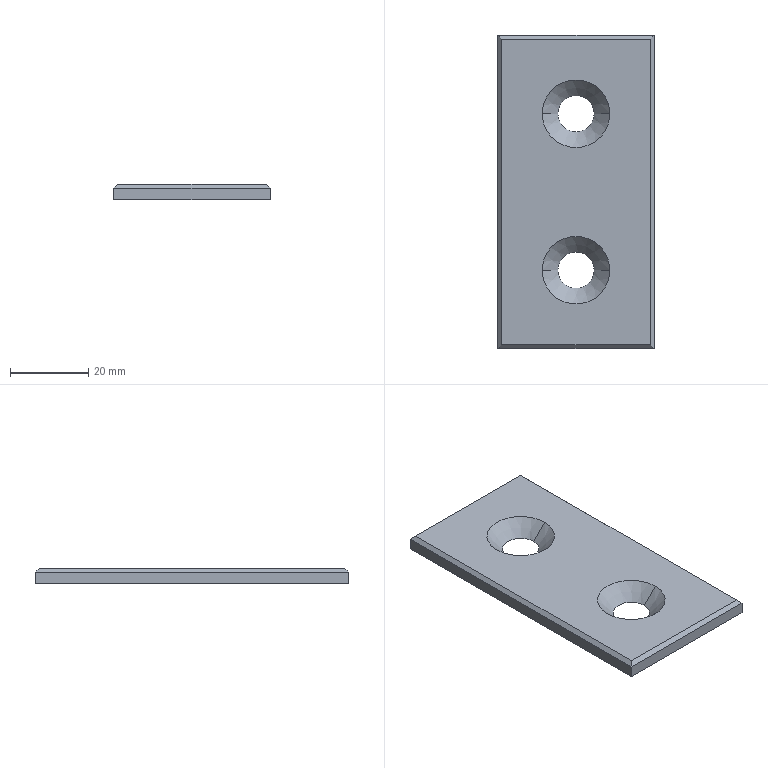Part | SolidWorks | features 3DProfileFeature 1, Chamfer 1, Extrusion 1, HoleWzd 1 | 1 solid | 14 faces | box 40 x 80 x 4 mm | volume 11536 mm3 | plane 10 | cone 4
STEP:
#1=CARTESIAN_POINT('',(-4.65,20.,-2.));
#2=VERTEX_POINT('',#1);
#3=CARTESIAN_POINT('',(4.65,20.,-2.));
#4=VERTEX_POINT('',#3);
#5=CARTESIAN_POINT('',(0.,20.,-2.));
#6=DIRECTION('',(0.,0.,1.));
#7=DIRECTION('',(1.,0.,0.));
#8=AXIS2_PLACEMENT_3D('',#5,#6,#7);
#9=CIRCLE('',#8,4.65);
#10=EDGE_CURVE('',#2,#4,#9,.T.);
#11=ORIENTED_EDGE('',*,*,#10,.F.);
#12=CARTESIAN_POINT('',(-8.65,20.,2.));
#13=VERTEX_POINT('',#12);
#14=CARTESIAN_POINT('',(-8.65,20.,2.));
#15=DIRECTION('',(-0.7071,0.,0.7071));
#16=VECTOR('',#15,1000.);
#17=LINE('',#14,#16);
#18=EDGE_CURVE('',#2,#13,#17,.T.);
#19=ORIENTED_EDGE('',*,*,#18,.T.);
#20=CARTESIAN_POINT('',(8.65,20.,2.));
#21=VERTEX_POINT('',#20);
#22=CARTESIAN_POINT('',(0.,20.,2.));
#23=DIRECTION('',(0.,0.,1.));
#24=DIRECTION('',(1.,0.,0.));
#25=AXIS2_PLACEMENT_3D('',#22,#23,#24);
#26=CIRCLE('',#25,8.65);
#27=EDGE_CURVE('',#13,#21,#26,.T.);
#28=ORIENTED_EDGE('',*,*,#27,.T.);
#29=CARTESIAN_POINT('',(8.65,20.,2.));
#30=DIRECTION('',(0.7071,0.,0.7071));
#31=VECTOR('',#30,1000.);
#32=LINE('',#29,#31);
#33=EDGE_CURVE('',#4,#21,#32,.T.);
#34=ORIENTED_EDGE('',*,*,#33,.F.);
#35=EDGE_LOOP('',(#11,#19,#28,#34));
#36=FACE_OUTER_BOUND('',#35,.T.);
#37=CARTESIAN_POINT('',(0.,20.,2.));
#38=DIRECTION('',(0.,0.,1.));
#39=DIRECTION('',(1.,0.,0.));
#40=AXIS2_PLACEMENT_3D('',#37,#38,#39);
#41=CONICAL_SURFACE('',#40,8.65,0.7854);
#42=ADVANCED_FACE('',(#36),#41,.F.);
#43=CARTESIAN_POINT('',(-4.65,-20.,-2.));
#44=VERTEX_POINT('',#43);
#45=CARTESIAN_POINT('',(4.65,-20.,-2.));
#46=VERTEX_POINT('',#45);
#47=CARTESIAN_POINT('',(0.,-20.,-2.));
#48=DIRECTION('',(0.,0.,1.));
#49=DIRECTION('',(1.,0.,0.));
#50=AXIS2_PLACEMENT_3D('',#47,#48,#49);
#51=CIRCLE('',#50,4.65);
#52=EDGE_CURVE('',#44,#46,#51,.T.);
#53=ORIENTED_EDGE('',*,*,#52,.F.);
#54=CARTESIAN_POINT('',(-8.65,-20.,2.));
#55=VERTEX_POINT('',#54);
#56=CARTESIAN_POINT('',(-8.65,-20.,2.));
#57=DIRECTION('',(-0.7071,0.,0.7071));
#58=VECTOR('',#57,1000.);
#59=LINE('',#56,#58);
#60=EDGE_CURVE('',#44,#55,#59,.T.);
#61=ORIENTED_EDGE('',*,*,#60,.T.);
#62=CARTESIAN_POINT('',(8.65,-20.,2.));
#63=VERTEX_POINT('',#62);
#64=CARTESIAN_POINT('',(0.,-20.,2.));
#65=DIRECTION('',(0.,0.,1.));
#66=DIRECTION('',(1.,0.,0.));
#67=AXIS2_PLACEMENT_3D('',#64,#65,#66);
#68=CIRCLE('',#67,8.65);
#69=EDGE_CURVE('',#55,#63,#68,.T.);
#70=ORIENTED_EDGE('',*,*,#69,.T.);
#71=CARTESIAN_POINT('',(8.65,-20.,2.));
#72=DIRECTION('',(0.7071,0.,0.7071));
#73=VECTOR('',#72,1000.);
#74=LINE('',#71,#73);
#75=EDGE_CURVE('',#46,#63,#74,.T.);
#76=ORIENTED_EDGE('',*,*,#75,.F.);
#77=EDGE_LOOP('',(#53,#61,#70,#76));
#78=FACE_OUTER_BOUND('',#77,.T.);
#79=CARTESIAN_POINT('',(0.,-20.,2.));
#80=DIRECTION('',(0.,0.,1.));
#81=DIRECTION('',(1.,0.,0.));
#82=AXIS2_PLACEMENT_3D('',#79,#80,#81);
#83=CONICAL_SURFACE('',#82,8.65,0.7854);
#84=ADVANCED_FACE('',(#78),#83,.F.);
#85=CARTESIAN_POINT('',(20.,40.,1.));
#86=VERTEX_POINT('',#85);
#87=CARTESIAN_POINT('',(20.,40.,-2.));
#88=VERTEX_POINT('',#87);
#89=CARTESIAN_POINT('',(20.,40.,2.));
#90=DIRECTION('',(0.,0.,-1.));
#91=VECTOR('',#90,1000.);
#92=LINE('',#89,#91);
#93=EDGE_CURVE('',#86,#88,#92,.T.);
#94=ORIENTED_EDGE('',*,*,#93,.F.);
#95=CARTESIAN_POINT('',(20.,-40.,1.));
#96=VERTEX_POINT('',#95);
#97=CARTESIAN_POINT('',(20.,-40.,1.));
#98=DIRECTION('',(0.,-1.,0.));
#99=VECTOR('',#98,1000.);
#100=LINE('',#97,#99);
#101=EDGE_CURVE('',#86,#96,#100,.T.);
#102=ORIENTED_EDGE('',*,*,#101,.T.);
#103=CARTESIAN_POINT('',(20.,-40.,-2.));
#104=VERTEX_POINT('',#103);
#105=CARTESIAN_POINT('',(20.,-40.,2.));
#106=DIRECTION('',(0.,0.,-1.));
#107=VECTOR('',#106,1000.);
#108=LINE('',#105,#107);
#109=EDGE_CURVE('',#96,#104,#108,.T.);
#110=ORIENTED_EDGE('',*,*,#109,.T.);
#111=CARTESIAN_POINT('',(20.,40.,-2.));
#112=DIRECTION('',(0.,1.,0.));
#113=VECTOR('',#112,1000.);
#114=LINE('',#111,#113);
#115=EDGE_CURVE('',#104,#88,#114,.T.);
#116=ORIENTED_EDGE('',*,*,#115,.T.);
#117=EDGE_LOOP('',(#94,#102,#110,#116));
#118=FACE_OUTER_BOUND('',#117,.T.);
#119=CARTESIAN_POINT('',(20.,40.,2.));
#120=DIRECTION('',(-1.,0.,0.));
#121=DIRECTION('',(0.,-1.,0.));
#122=AXIS2_PLACEMENT_3D('',#119,#120,#121);
#123=PLANE('',#122);
#124=ADVANCED_FACE('',(#118),#123,.F.);
#125=CARTESIAN_POINT('',(-20.,40.,1.));
#126=VERTEX_POINT('',#125);
#127=CARTESIAN_POINT('',(-20.,40.,-2.));
#128=VERTEX_POINT('',#127);
#129=CARTESIAN_POINT('',(-20.,40.,2.));
#130=DIRECTION('',(0.,0.,-1.));
#131=VECTOR('',#130,1000.);
#132=LINE('',#129,#131);
#133=EDGE_CURVE('',#126,#128,#132,.T.);
#134=ORIENTED_EDGE('',*,*,#133,.F.);
#135=CARTESIAN_POINT('',(20.,40.,1.));
#136=DIRECTION('',(1.,0.,0.));
#137=VECTOR('',#136,1000.);
#138=LINE('',#135,#137);
#139=EDGE_CURVE('',#126,#86,#138,.T.);
#140=ORIENTED_EDGE('',*,*,#139,.T.);
#141=ORIENTED_EDGE('',*,*,#93,.T.);
#142=CARTESIAN_POINT('',(-20.,40.,-2.));
#143=DIRECTION('',(-1.,0.,0.));
#144=VECTOR('',#143,1000.);
#145=LINE('',#142,#144);
#146=EDGE_CURVE('',#88,#128,#145,.T.);
#147=ORIENTED_EDGE('',*,*,#146,.T.);
#148=EDGE_LOOP('',(#134,#140,#141,#147));
#149=FACE_OUTER_BOUND('',#148,.T.);
#150=CARTESIAN_POINT('',(-20.,40.,2.));
#151=DIRECTION('',(0.,-1.,0.));
#152=DIRECTION('',(0.,0.,-1.));
#153=AXIS2_PLACEMENT_3D('',#150,#151,#152);
#154=PLANE('',#153);
#155=ADVANCED_FACE('',(#149),#154,.F.);
#156=CARTESIAN_POINT('',(-20.,-40.,1.));
#157=VERTEX_POINT('',#156);
#158=CARTESIAN_POINT('',(-20.,-40.,-2.));
#159=VERTEX_POINT('',#158);
#160=CARTESIAN_POINT('',(-20.,-40.,2.));
#161=DIRECTION('',(0.,0.,-1.));
#162=VECTOR('',#161,1000.);
#163=LINE('',#160,#162);
#164=EDGE_CURVE('',#157,#159,#163,.T.);
#165=ORIENTED_EDGE('',*,*,#164,.F.);
#166=CARTESIAN_POINT('',(-20.,40.,1.));
#167=DIRECTION('',(0.,1.,0.));
#168=VECTOR('',#167,1000.);
#169=LINE('',#166,#168);
#170=EDGE_CURVE('',#157,#126,#169,.T.);
#171=ORIENTED_EDGE('',*,*,#170,.T.);
#172=ORIENTED_EDGE('',*,*,#133,.T.);
#173=CARTESIAN_POINT('',(-20.,40.,-2.));
#174=DIRECTION('',(0.,-1.,0.));
#175=VECTOR('',#174,1000.);
#176=LINE('',#173,#175);
#177=EDGE_CURVE('',#128,#159,#176,.T.);
#178=ORIENTED_EDGE('',*,*,#177,.T.);
#179=EDGE_LOOP('',(#165,#171,#172,#178));
#180=FACE_OUTER_BOUND('',#179,.T.);
#181=CARTESIAN_POINT('',(-20.,40.,2.));
#182=DIRECTION('',(1.,0.,0.));
#183=DIRECTION('',(0.,1.,0.));
#184=AXIS2_PLACEMENT_3D('',#181,#182,#183);
#185=PLANE('',#184);
#186=ADVANCED_FACE('',(#180),#185,.F.);
#187=ORIENTED_EDGE('',*,*,#109,.F.);
#188=CARTESIAN_POINT('',(-20.,-40.,1.));
#189=DIRECTION('',(-1.,0.,0.));
#190=VECTOR('',#189,1000.);
#191=LINE('',#188,#190);
#192=EDGE_CURVE('',#96,#157,#191,.T.);
#193=ORIENTED_EDGE('',*,*,#192,.T.);
#194=ORIENTED_EDGE('',*,*,#164,.T.);
#195=CARTESIAN_POINT('',(-20.,-40.,-2.));
#196=DIRECTION('',(1.,0.,0.));
#197=VECTOR('',#196,1000.);
#198=LINE('',#195,#197);
#199=EDGE_CURVE('',#159,#104,#198,.T.);
#200=ORIENTED_EDGE('',*,*,#199,.T.);
#201=EDGE_LOOP('',(#187,#193,#194,#200));
#202=FACE_OUTER_BOUND('',#201,.T.);
#203=CARTESIAN_POINT('',(-20.,-40.,2.));
#204=DIRECTION('',(0.,1.,0.));
#205=DIRECTION('',(0.,0.,1.));
#206=AXIS2_PLACEMENT_3D('',#203,#204,#205);
#207=PLANE('',#206);
#208=ADVANCED_FACE('',(#202),#207,.F.);
#209=CARTESIAN_POINT('',(-19.,39.,2.));
#210=VERTEX_POINT('',#209);
#211=CARTESIAN_POINT('',(-19.,-39.,2.));
#212=VERTEX_POINT('',#211);
#213=CARTESIAN_POINT('',(-19.,-40.,2.));
#214=DIRECTION('',(0.,-1.,0.));
#215=VECTOR('',#214,1000.);
#216=LINE('',#213,#215);
#217=EDGE_CURVE('',#210,#212,#216,.T.);
#218=ORIENTED_EDGE('',*,*,#217,.T.);
#219=CARTESIAN_POINT('',(19.,-39.,2.));
#220=VERTEX_POINT('',#219);
#221=CARTESIAN_POINT('',(20.,-39.,2.));
#222=DIRECTION('',(1.,0.,0.));
#223=VECTOR('',#222,1000.);
#224=LINE('',#221,#223);
#225=EDGE_CURVE('',#212,#220,#224,.T.);
#226=ORIENTED_EDGE('',*,*,#225,.T.);
#227=CARTESIAN_POINT('',(19.,39.,2.));
#228=VERTEX_POINT('',#227);
#229=CARTESIAN_POINT('',(19.,40.,2.));
#230=DIRECTION('',(0.,1.,0.));
#231=VECTOR('',#230,1000.);
#232=LINE('',#229,#231);
#233=EDGE_CURVE('',#220,#228,#232,.T.);
#234=ORIENTED_EDGE('',*,*,#233,.T.);
#235=CARTESIAN_POINT('',(-20.,39.,2.));
#236=DIRECTION('',(-1.,0.,0.));
#237=VECTOR('',#236,1000.);
#238=LINE('',#235,#237);
#239=EDGE_CURVE('',#228,#210,#238,.T.);
#240=ORIENTED_EDGE('',*,*,#239,.T.);
#241=EDGE_LOOP('',(#218,#226,#234,#240));
#242=FACE_OUTER_BOUND('',#241,.T.);
#243=CARTESIAN_POINT('',(0.,20.,2.));
#244=DIRECTION('',(0.,0.,1.));
#245=DIRECTION('',(1.,0.,0.));
#246=AXIS2_PLACEMENT_3D('',#243,#244,#245);
#247=CIRCLE('',#246,8.65);
#248=EDGE_CURVE('',#21,#13,#247,.T.);
#249=ORIENTED_EDGE('',*,*,#248,.F.);
#250=ORIENTED_EDGE('',*,*,#27,.F.);
#251=EDGE_LOOP('',(#249,#250));
#252=FACE_BOUND('',#251,.T.);
#253=CARTESIAN_POINT('',(0.,-20.,2.));
#254=DIRECTION('',(0.,0.,1.));
#255=DIRECTION('',(1.,0.,0.));
#256=AXIS2_PLACEMENT_3D('',#253,#254,#255);
#257=CIRCLE('',#256,8.65);
#258=EDGE_CURVE('',#63,#55,#257,.T.);
#259=ORIENTED_EDGE('',*,*,#258,.F.);
#260=ORIENTED_EDGE('',*,*,#69,.F.);
#261=EDGE_LOOP('',(#259,#260));
#262=FACE_BOUND('',#261,.T.);
#263=CARTESIAN_POINT('',(0.,0.,2.));
#264=DIRECTION('',(0.,0.,1.));
#265=DIRECTION('',(1.,0.,0.));
#266=AXIS2_PLACEMENT_3D('',#263,#264,#265);
#267=PLANE('',#266);
#268=ADVANCED_FACE('',(#242,#252,#262),#267,.T.);
#269=CARTESIAN_POINT('',(0.,20.,-2.));
#270=DIRECTION('',(0.,0.,1.));
#271=DIRECTION('',(1.,0.,0.));
#272=AXIS2_PLACEMENT_3D('',#269,#270,#271);
#273=CIRCLE('',#272,4.65);
#274=EDGE_CURVE('',#4,#2,#273,.T.);
#275=ORIENTED_EDGE('',*,*,#274,.T.);
#276=ORIENTED_EDGE('',*,*,#10,.T.);
#277=EDGE_LOOP('',(#275,#276));
#278=FACE_BOUND('',#277,.T.);
#279=CARTESIAN_POINT('',(0.,-20.,-2.));
#280=DIRECTION('',(0.,0.,1.));
#281=DIRECTION('',(1.,0.,0.));
#282=AXIS2_PLACEMENT_3D('',#279,#280,#281);
#283=CIRCLE('',#282,4.65);
#284=EDGE_CURVE('',#46,#44,#283,.T.);
#285=ORIENTED_EDGE('',*,*,#284,.T.);
#286=ORIENTED_EDGE('',*,*,#52,.T.);
#287=EDGE_LOOP('',(#285,#286));
#288=FACE_BOUND('',#287,.T.);
#289=ORIENTED_EDGE('',*,*,#115,.F.);
#290=ORIENTED_EDGE('',*,*,#199,.F.);
#291=ORIENTED_EDGE('',*,*,#177,.F.);
#292=ORIENTED_EDGE('',*,*,#146,.F.);
#293=EDGE_LOOP('',(#289,#290,#291,#292));
#294=FACE_OUTER_BOUND('',#293,.T.);
#295=CARTESIAN_POINT('',(0.,0.,-2.));
#296=DIRECTION('',(0.,0.,1.));
#297=DIRECTION('',(1.,0.,0.));
#298=AXIS2_PLACEMENT_3D('',#295,#296,#297);
#299=PLANE('',#298);
#300=ADVANCED_FACE('',(#278,#288,#294),#299,.F.);
#301=ORIENTED_EDGE('',*,*,#60,.F.);
#302=ORIENTED_EDGE('',*,*,#284,.F.);
#303=ORIENTED_EDGE('',*,*,#75,.T.);
#304=ORIENTED_EDGE('',*,*,#258,.T.);
#305=EDGE_LOOP('',(#301,#302,#303,#304));
#306=FACE_OUTER_BOUND('',#305,.T.);
#307=CARTESIAN_POINT('',(0.,-20.,2.));
#308=DIRECTION('',(0.,0.,1.));
#309=DIRECTION('',(1.,0.,0.));
#310=AXIS2_PLACEMENT_3D('',#307,#308,#309);
#311=CONICAL_SURFACE('',#310,8.65,0.7854);
#312=ADVANCED_FACE('',(#306),#311,.F.);
#313=ORIENTED_EDGE('',*,*,#18,.F.);
#314=ORIENTED_EDGE('',*,*,#274,.F.);
#315=ORIENTED_EDGE('',*,*,#33,.T.);
#316=ORIENTED_EDGE('',*,*,#248,.T.);
#317=EDGE_LOOP('',(#313,#314,#315,#316));
#318=FACE_OUTER_BOUND('',#317,.T.);
#319=CARTESIAN_POINT('',(0.,20.,2.));
#320=DIRECTION('',(0.,0.,1.));
#321=DIRECTION('',(1.,0.,0.));
#322=AXIS2_PLACEMENT_3D('',#319,#320,#321);
#323=CONICAL_SURFACE('',#322,8.65,0.7854);
#324=ADVANCED_FACE('',(#318),#323,.F.);
#325=CARTESIAN_POINT('',(6.,26.,15.));
#326=DIRECTION('',(-0.5774,-0.5774,0.5774));
#327=VECTOR('',#326,1000.);
#328=LINE('',#325,#327);
#329=EDGE_CURVE('',#86,#228,#328,.T.);
#330=ORIENTED_EDGE('',*,*,#329,.F.);
#331=ORIENTED_EDGE('',*,*,#139,.F.);
#332=CARTESIAN_POINT('',(-12.667,32.667,8.333));
#333=DIRECTION('',(-0.5774,0.5774,-0.5774));
#334=VECTOR('',#333,1000.);
#335=LINE('',#332,#334);
#336=EDGE_CURVE('',#210,#126,#335,.T.);
#337=ORIENTED_EDGE('',*,*,#336,.F.);
#338=ORIENTED_EDGE('',*,*,#239,.F.);
#339=EDGE_LOOP('',(#330,#331,#337,#338));
#340=FACE_OUTER_BOUND('',#339,.T.);
#341=CARTESIAN_POINT('',(0.,39.,2.));
#342=DIRECTION('',(0.,0.7071,0.7071));
#343=DIRECTION('',(1.,0.,0.));
#344=AXIS2_PLACEMENT_3D('',#341,#342,#343);
#345=PLANE('',#344);
#346=ADVANCED_FACE('',(#340),#345,.T.);
#347=ORIENTED_EDGE('',*,*,#336,.T.);
#348=ORIENTED_EDGE('',*,*,#170,.F.);
#349=CARTESIAN_POINT('',(-6.,-26.,15.));
#350=DIRECTION('',(-0.5774,-0.5774,-0.5774));
#351=VECTOR('',#350,1000.);
#352=LINE('',#349,#351);
#353=EDGE_CURVE('',#212,#157,#352,.T.);
#354=ORIENTED_EDGE('',*,*,#353,.F.);
#355=ORIENTED_EDGE('',*,*,#217,.F.);
#356=EDGE_LOOP('',(#347,#348,#354,#355));
#357=FACE_OUTER_BOUND('',#356,.T.);
#358=CARTESIAN_POINT('',(-19.,0.,2.));
#359=DIRECTION('',(-0.7071,0.,0.7071));
#360=DIRECTION('',(0.,1.,0.));
#361=AXIS2_PLACEMENT_3D('',#358,#359,#360);
#362=PLANE('',#361);
#363=ADVANCED_FACE('',(#357),#362,.T.);
#364=ORIENTED_EDGE('',*,*,#329,.T.);
#365=ORIENTED_EDGE('',*,*,#233,.F.);
#366=CARTESIAN_POINT('',(6.,-26.,15.));
#367=DIRECTION('',(-0.5774,0.5774,0.5774));
#368=VECTOR('',#367,1000.);
#369=LINE('',#366,#368);
#370=EDGE_CURVE('',#96,#220,#369,.T.);
#371=ORIENTED_EDGE('',*,*,#370,.F.);
#372=ORIENTED_EDGE('',*,*,#101,.F.);
#373=EDGE_LOOP('',(#364,#365,#371,#372));
#374=FACE_OUTER_BOUND('',#373,.T.);
#375=CARTESIAN_POINT('',(19.,0.,2.));
#376=DIRECTION('',(0.7071,0.,0.7071));
#377=DIRECTION('',(0.,-1.,0.));
#378=AXIS2_PLACEMENT_3D('',#375,#376,#377);
#379=PLANE('',#378);
#380=ADVANCED_FACE('',(#374),#379,.T.);
#381=ORIENTED_EDGE('',*,*,#353,.T.);
#382=ORIENTED_EDGE('',*,*,#192,.F.);
#383=ORIENTED_EDGE('',*,*,#370,.T.);
#384=ORIENTED_EDGE('',*,*,#225,.F.);
#385=EDGE_LOOP('',(#381,#382,#383,#384));
#386=FACE_OUTER_BOUND('',#385,.T.);
#387=CARTESIAN_POINT('',(0.,-39.,2.));
#388=DIRECTION('',(0.,-0.7071,0.7071));
#389=DIRECTION('',(-1.,0.,0.));
#390=AXIS2_PLACEMENT_3D('',#387,#388,#389);
#391=PLANE('',#390);
#392=ADVANCED_FACE('',(#386),#391,.T.);
#393=CLOSED_SHELL('',(#42,#84,#124,#155,#186,#208,#268,#300,#312,#324,#346,#363,#380,#392));
#394=MANIFOLD_SOLID_BREP('',#393);
#395=CARTESIAN_POINT('',(0.,0.,0.));
#396=DIRECTION('',(0.,0.,1.));
#397=DIRECTION('',(1.,0.,0.));
#398=AXIS2_PLACEMENT_3D('',#395,#396,#397);
#399=(LENGTH_UNIT()NAMED_UNIT(*)SI_UNIT(.MILLI.,.METRE.));
#400=UNCERTAINTY_MEASURE_WITH_UNIT(LENGTH_MEASURE(0.00001),#399,'','');
#401=(NAMED_UNIT(*)PLANE_ANGLE_UNIT()SI_UNIT($,.RADIAN.));
#402=(NAMED_UNIT(*)SI_UNIT($,.STERADIAN.)SOLID_ANGLE_UNIT());
#403=(GEOMETRIC_REPRESENTATION_CONTEXT(3)GLOBAL_UNCERTAINTY_ASSIGNED_CONTEXT((#400))GLOBAL_UNIT_ASSIGNED_CONTEXT((#399,#401,#402))REPRESENTATION_CONTEXT('',''));
#404=ADVANCED_BREP_SHAPE_REPRESENTATION('',(#394,#398),#403);